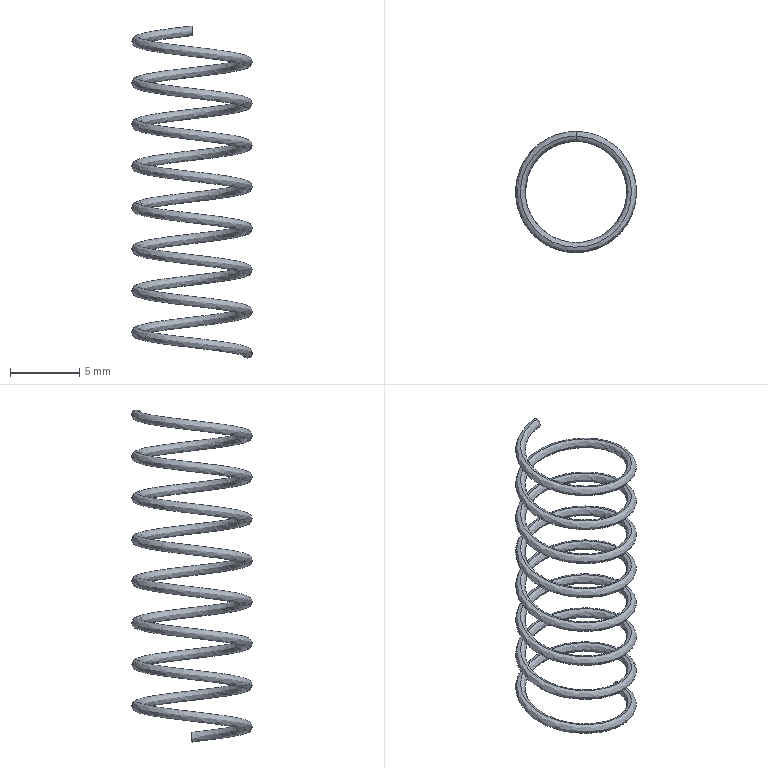Part | STEP file | Spring-hub step test | 1 solid | 4 faces | box 8.7 x 8.7 x 23.95 mm | volume 74.991 mm3 | spline 2 | plane 2